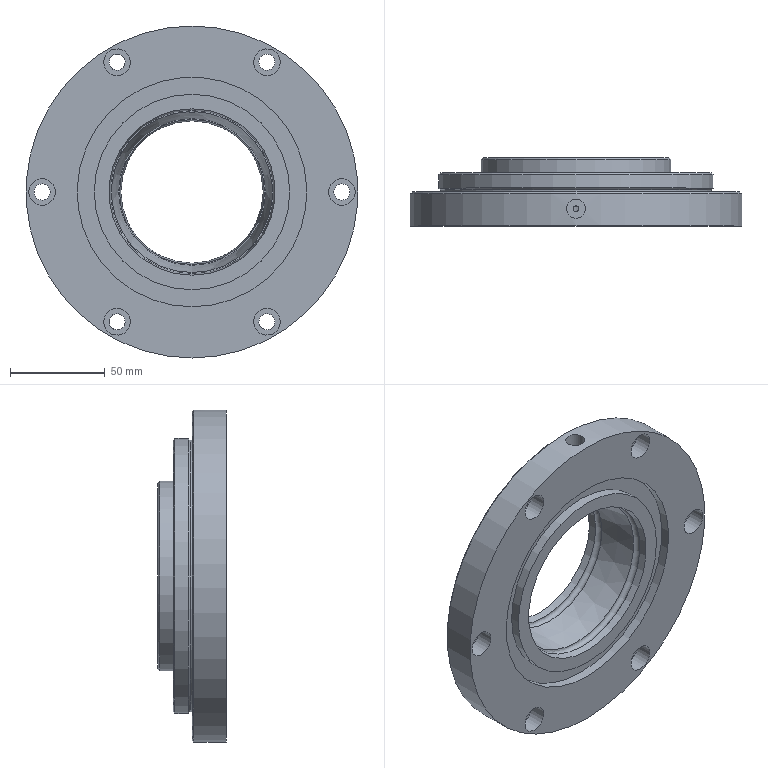Part | NX | features IDENTICAL INSTANCE OUTPUT 5, Instance Feature 5, DATUM_CSYS 3, CBORE_HOLE 2, HOLE PACKAGE 2, SKETCH 2, CHAMFER 1, MASTER SNAPSHOT BODY 1, Pattern Feature 1, SWP104 1 | 1 solid | 44 faces | box 175 x 36 x 175 mm | volume 439524 mm3 | cylinder 20 | plane 14 | cone 8 | torus 2 | commonest cylinder face diameters 8.5 x6 14 x6 3 x1 10 x1 100 x1 103 x1
STEP:
#1=CARTESIAN_POINT('',(0.,0.,-43.848));
#2=VERTEX_POINT('',#1);
#3=CARTESIAN_POINT('',(0.,0.,0.));
#4=DIRECTION('',(0.,-1.,0.));
#5=DIRECTION('',(0.,0.,-1.));
#6=AXIS2_PLACEMENT_3D('',#3,#4,#5);
#7=CIRCLE('',#6,43.848);
#8=EDGE_CURVE('',#2,#2,#7,.T.);
#9=ORIENTED_EDGE('',*,*,#8,.F.);
#10=EDGE_LOOP('',(#9));
#11=FACE_BOUND('',#10,.T.);
#12=CARTESIAN_POINT('',(0.,0.,-51.5));
#13=VERTEX_POINT('',#12);
#14=CARTESIAN_POINT('',(0.,0.,0.));
#15=DIRECTION('',(0.,-1.,0.));
#16=DIRECTION('',(0.,0.,-1.));
#17=AXIS2_PLACEMENT_3D('',#14,#15,#16);
#18=CIRCLE('',#17,51.5);
#19=EDGE_CURVE('',#13,#13,#18,.T.);
#20=ORIENTED_EDGE('',*,*,#19,.T.);
#21=EDGE_LOOP('',(#20));
#22=FACE_BOUND('',#21,.T.);
#23=CARTESIAN_POINT('',(0.,0.,51.5));
#24=DIRECTION('',(0.,1.,0.));
#25=DIRECTION('',(0.,0.,1.));
#26=AXIS2_PLACEMENT_3D('',#23,#24,#25);
#27=PLANE('',#26);
#28=ADVANCED_FACE('',(#11,#22),#27,.F.);
#29=CARTESIAN_POINT('',(0.,4.,-43.142));
#30=VERTEX_POINT('',#29);
#31=CARTESIAN_POINT('',(0.,4.,0.));
#32=DIRECTION('',(0.,-1.,0.));
#33=DIRECTION('',(0.,0.,-1.));
#34=AXIS2_PLACEMENT_3D('',#31,#32,#33);
#35=CIRCLE('',#34,43.142);
#36=EDGE_CURVE('',#30,#30,#35,.T.);
#37=ORIENTED_EDGE('',*,*,#36,.F.);
#38=EDGE_LOOP('',(#37));
#39=FACE_BOUND('',#38,.T.);
#40=ORIENTED_EDGE('',*,*,#8,.T.);
#41=EDGE_LOOP('',(#40));
#42=FACE_BOUND('',#41,.T.);
#43=CARTESIAN_POINT('',(0.,0.,0.));
#44=DIRECTION('',(0.,-1.,0.));
#45=DIRECTION('',(0.,0.,-1.));
#46=AXIS2_PLACEMENT_3D('',#43,#44,#45);
#47=CONICAL_SURFACE('',#46,43.848,0.1745);
#48=ADVANCED_FACE('',(#39,#42),#47,.F.);
#49=CARTESIAN_POINT('',(-1.061,7.939,42.435));
#50=VERTEX_POINT('',#49);
#51=CARTESIAN_POINT('',(1.061,7.939,42.435));
#52=VERTEX_POINT('',#51);
#53=CARTESIAN_POINT('',(0.,7.939,0.));
#54=DIRECTION('',(0.,-1.,0.));
#55=DIRECTION('',(0.,0.,-1.));
#56=AXIS2_PLACEMENT_3D('',#53,#54,#55);
#57=CIRCLE('',#56,42.448);
#58=EDGE_CURVE('',#50,#52,#57,.T.);
#59=ORIENTED_EDGE('',*,*,#58,.F.);
#60=CARTESIAN_POINT('',(-1.061,7.939,42.435));
#61=CARTESIAN_POINT('',(-1.128,8.006,42.814));
#62=CARTESIAN_POINT('',(-1.087,7.877,43.66));
#63=CARTESIAN_POINT('',(-0.2099,7.412,44.182));
#64=CARTESIAN_POINT('',(0.5847,7.583,43.99));
#65=CARTESIAN_POINT('',(1.08,7.916,43.444));
#66=CARTESIAN_POINT('',(1.128,8.006,42.814));
#67=CARTESIAN_POINT('',(1.061,7.939,42.435));
#68=B_SPLINE_CURVE_WITH_KNOTS('',3,(#60,#61,#62,#63,#64,#65,#66,#67),.UNSPECIFIED.,.F.,.F.,(4,1,1,1,1,4),(0.0008258,0.001986,0.003146,0.003726,0.004307,0.005467),.UNSPECIFIED.);
#69=EDGE_CURVE('',#50,#52,#68,.T.);
#70=ORIENTED_EDGE('',*,*,#69,.T.);
#71=EDGE_LOOP('',(#59,#70));
#72=FACE_BOUND('',#71,.T.);
#73=ORIENTED_EDGE('',*,*,#36,.T.);
#74=EDGE_LOOP('',(#73));
#75=FACE_BOUND('',#74,.T.);
#76=CARTESIAN_POINT('',(0.,5.97,0.));
#77=DIRECTION('',(0.,-1.,0.));
#78=DIRECTION('',(0.,0.,-1.));
#79=AXIS2_PLACEMENT_3D('',#76,#77,#78);
#80=TOROIDAL_SURFACE('',#79,42.795,2.);
#81=ADVANCED_FACE('',(#72,#75),#80,.F.);
#82=CARTESIAN_POINT('',(0.,28.061,-38.9));
#83=VERTEX_POINT('',#82);
#84=CARTESIAN_POINT('',(0.,28.061,0.));
#85=DIRECTION('',(0.,-1.,0.));
#86=DIRECTION('',(0.,0.,-1.));
#87=AXIS2_PLACEMENT_3D('',#84,#85,#86);
#88=CIRCLE('',#87,38.9);
#89=EDGE_CURVE('',#83,#83,#88,.T.);
#90=ORIENTED_EDGE('',*,*,#89,.F.);
#91=EDGE_LOOP('',(#90));
#92=FACE_BOUND('',#91,.T.);
#93=ORIENTED_EDGE('',*,*,#58,.T.);
#94=CARTESIAN_POINT('',(1.061,7.939,42.435));
#95=CARTESIAN_POINT('',(1.481,8.359,42.35));
#96=CARTESIAN_POINT('',(1.747,9.702,42.103));
#97=CARTESIAN_POINT('',(0.001721,10.899,41.943));
#98=CARTESIAN_POINT('',(-1.747,9.703,42.103));
#99=CARTESIAN_POINT('',(-1.481,8.359,42.35));
#100=CARTESIAN_POINT('',(-1.061,7.939,42.435));
#101=B_SPLINE_CURVE_WITH_KNOTS('',3,(#94,#95,#96,#97,#98,#99,#100),.UNSPECIFIED.,.F.,.F.,(4,1,1,1,4),(0.000000282,0.001775,0.003549,0.005324,0.007098),.UNSPECIFIED.);
#102=EDGE_CURVE('',#52,#50,#101,.T.);
#103=ORIENTED_EDGE('',*,*,#102,.T.);
#104=EDGE_LOOP('',(#93,#103));
#105=FACE_BOUND('',#104,.T.);
#106=CARTESIAN_POINT('',(0.,7.939,0.));
#107=DIRECTION('',(0.,-1.,0.));
#108=DIRECTION('',(0.,0.,-1.));
#109=AXIS2_PLACEMENT_3D('',#106,#107,#108);
#110=CONICAL_SURFACE('',#109,42.448,0.1745);
#111=ADVANCED_FACE('',(#92,#105),#110,.F.);
#112=CARTESIAN_POINT('',(0.,32.,-38.205));
#113=VERTEX_POINT('',#112);
#114=CARTESIAN_POINT('',(0.,32.,0.));
#115=DIRECTION('',(0.,-1.,0.));
#116=DIRECTION('',(0.,0.,-1.));
#117=AXIS2_PLACEMENT_3D('',#114,#115,#116);
#118=CIRCLE('',#117,38.205);
#119=EDGE_CURVE('',#113,#113,#118,.T.);
#120=ORIENTED_EDGE('',*,*,#119,.F.);
#121=EDGE_LOOP('',(#120));
#122=FACE_BOUND('',#121,.T.);
#123=ORIENTED_EDGE('',*,*,#89,.T.);
#124=EDGE_LOOP('',(#123));
#125=FACE_BOUND('',#124,.T.);
#126=CARTESIAN_POINT('',(0.,30.03,0.));
#127=DIRECTION('',(0.,-1.,0.));
#128=DIRECTION('',(0.,0.,-1.));
#129=AXIS2_PLACEMENT_3D('',#126,#127,#128);
#130=TOROIDAL_SURFACE('',#129,38.553,2.);
#131=ADVANCED_FACE('',(#122,#125),#130,.F.);
#132=CARTESIAN_POINT('',(0.,36.,-37.5));
#133=VERTEX_POINT('',#132);
#134=CARTESIAN_POINT('',(0.,36.,0.));
#135=DIRECTION('',(0.,-1.,0.));
#136=DIRECTION('',(0.,0.,-1.));
#137=AXIS2_PLACEMENT_3D('',#134,#135,#136);
#138=CIRCLE('',#137,37.5);
#139=EDGE_CURVE('',#133,#133,#138,.T.);
#140=ORIENTED_EDGE('',*,*,#139,.F.);
#141=EDGE_LOOP('',(#140));
#142=FACE_BOUND('',#141,.T.);
#143=ORIENTED_EDGE('',*,*,#119,.T.);
#144=EDGE_LOOP('',(#143));
#145=FACE_BOUND('',#144,.T.);
#146=CARTESIAN_POINT('',(0.,32.,0.));
#147=DIRECTION('',(0.,-1.,0.));
#148=DIRECTION('',(0.,0.,-1.));
#149=AXIS2_PLACEMENT_3D('',#146,#147,#148);
#150=CONICAL_SURFACE('',#149,38.205,0.1745);
#151=ADVANCED_FACE('',(#142,#145),#150,.F.);
#152=CARTESIAN_POINT('',(0.,36.,-49.));
#153=VERTEX_POINT('',#152);
#154=CARTESIAN_POINT('',(0.,36.,0.));
#155=DIRECTION('',(0.,-1.,0.));
#156=DIRECTION('',(0.,0.,-1.));
#157=AXIS2_PLACEMENT_3D('',#154,#155,#156);
#158=CIRCLE('',#157,49.);
#159=EDGE_CURVE('',#153,#153,#158,.F.);
#160=ORIENTED_EDGE('',*,*,#159,.T.);
#161=EDGE_LOOP('',(#160));
#162=FACE_BOUND('',#161,.T.);
#163=ORIENTED_EDGE('',*,*,#139,.T.);
#164=EDGE_LOOP('',(#163));
#165=FACE_BOUND('',#164,.T.);
#166=CARTESIAN_POINT('',(0.,36.,37.5));
#167=DIRECTION('',(0.,-1.,0.));
#168=DIRECTION('',(0.,0.,-1.));
#169=AXIS2_PLACEMENT_3D('',#166,#167,#168);
#170=PLANE('',#169);
#171=ADVANCED_FACE('',(#162,#165),#170,.F.);
#172=CARTESIAN_POINT('',(0.,35.,-50.));
#173=VERTEX_POINT('',#172);
#174=CARTESIAN_POINT('',(0.,35.,0.));
#175=DIRECTION('',(0.,-1.,0.));
#176=DIRECTION('',(0.,0.,-1.));
#177=AXIS2_PLACEMENT_3D('',#174,#175,#176);
#178=CIRCLE('',#177,50.);
#179=EDGE_CURVE('',#173,#173,#178,.T.);
#180=ORIENTED_EDGE('',*,*,#179,.T.);
#181=EDGE_LOOP('',(#180));
#182=FACE_BOUND('',#181,.T.);
#183=CARTESIAN_POINT('',(0.,28.,-50.));
#184=VERTEX_POINT('',#183);
#185=CARTESIAN_POINT('',(0.,28.,0.));
#186=DIRECTION('',(0.,-1.,0.));
#187=DIRECTION('',(0.,0.,-1.));
#188=AXIS2_PLACEMENT_3D('',#185,#186,#187);
#189=CIRCLE('',#188,50.);
#190=EDGE_CURVE('',#184,#184,#189,.T.);
#191=ORIENTED_EDGE('',*,*,#190,.F.);
#192=EDGE_LOOP('',(#191));
#193=FACE_BOUND('',#192,.T.);
#194=CARTESIAN_POINT('',(0.,0.,0.));
#195=DIRECTION('',(0.,-1.,0.));
#196=DIRECTION('',(0.,0.,-1.));
#197=AXIS2_PLACEMENT_3D('',#194,#195,#196);
#198=CYLINDRICAL_SURFACE('',#197,50.);
#199=ADVANCED_FACE('',(#182,#193),#198,.T.);
#200=CARTESIAN_POINT('',(0.,28.,-71.5));
#201=VERTEX_POINT('',#200);
#202=CARTESIAN_POINT('',(0.,28.,0.));
#203=DIRECTION('',(0.,-1.,0.));
#204=DIRECTION('',(0.,0.,-1.));
#205=AXIS2_PLACEMENT_3D('',#202,#203,#204);
#206=CIRCLE('',#205,71.5);
#207=EDGE_CURVE('',#201,#201,#206,.F.);
#208=ORIENTED_EDGE('',*,*,#207,.T.);
#209=EDGE_LOOP('',(#208));
#210=FACE_BOUND('',#209,.T.);
#211=ORIENTED_EDGE('',*,*,#190,.T.);
#212=EDGE_LOOP('',(#211));
#213=FACE_BOUND('',#212,.T.);
#214=CARTESIAN_POINT('',(0.,28.,50.));
#215=DIRECTION('',(0.,-1.,0.));
#216=DIRECTION('',(0.,0.,-1.));
#217=AXIS2_PLACEMENT_3D('',#214,#215,#216);
#218=PLANE('',#217);
#219=ADVANCED_FACE('',(#210,#213),#218,.F.);
#220=CARTESIAN_POINT('',(0.,27.,-72.5));
#221=VERTEX_POINT('',#220);
#222=CARTESIAN_POINT('',(0.,27.,0.));
#223=DIRECTION('',(0.,-1.,0.));
#224=DIRECTION('',(0.,0.,-1.));
#225=AXIS2_PLACEMENT_3D('',#222,#223,#224);
#226=CIRCLE('',#225,72.5);
#227=EDGE_CURVE('',#221,#221,#226,.T.);
#228=ORIENTED_EDGE('',*,*,#227,.T.);
#229=EDGE_LOOP('',(#228));
#230=FACE_BOUND('',#229,.T.);
#231=CARTESIAN_POINT('',(0.,20.,-72.5));
#232=VERTEX_POINT('',#231);
#233=CARTESIAN_POINT('',(0.,20.,0.));
#234=DIRECTION('',(0.,-1.,0.));
#235=DIRECTION('',(0.,0.,-1.));
#236=AXIS2_PLACEMENT_3D('',#233,#234,#235);
#237=CIRCLE('',#236,72.5);
#238=EDGE_CURVE('',#232,#232,#237,.T.);
#239=ORIENTED_EDGE('',*,*,#238,.F.);
#240=EDGE_LOOP('',(#239));
#241=FACE_BOUND('',#240,.T.);
#242=CARTESIAN_POINT('',(0.,0.,0.));
#243=DIRECTION('',(0.,-1.,0.));
#244=DIRECTION('',(0.,0.,-1.));
#245=AXIS2_PLACEMENT_3D('',#242,#243,#244);
#246=CYLINDRICAL_SURFACE('',#245,72.5);
#247=ADVANCED_FACE('',(#230,#241),#246,.T.);
#248=CARTESIAN_POINT('',(0.,19.,-71.5));
#249=VERTEX_POINT('',#248);
#250=CARTESIAN_POINT('',(0.,19.,0.));
#251=DIRECTION('',(0.,-1.,0.));
#252=DIRECTION('',(0.,0.,-1.));
#253=AXIS2_PLACEMENT_3D('',#250,#251,#252);
#254=CIRCLE('',#253,71.5);
#255=EDGE_CURVE('',#249,#249,#254,.T.);
#256=ORIENTED_EDGE('',*,*,#255,.F.);
#257=EDGE_LOOP('',(#256));
#258=FACE_BOUND('',#257,.T.);
#259=ORIENTED_EDGE('',*,*,#238,.T.);
#260=EDGE_LOOP('',(#259));
#261=FACE_BOUND('',#260,.T.);
#262=CARTESIAN_POINT('',(0.,20.,0.));
#263=DIRECTION('',(0.,1.,0.));
#264=DIRECTION('',(0.,0.,1.));
#265=AXIS2_PLACEMENT_3D('',#262,#263,#264);
#266=CONICAL_SURFACE('',#265,72.5,0.7854);
#267=ADVANCED_FACE('',(#258,#261),#266,.T.);
#268=CARTESIAN_POINT('',(0.,17.,-71.5));
#269=VERTEX_POINT('',#268);
#270=CARTESIAN_POINT('',(0.,17.,0.));
#271=DIRECTION('',(0.,-1.,0.));
#272=DIRECTION('',(0.,0.,-1.));
#273=AXIS2_PLACEMENT_3D('',#270,#271,#272);
#274=CIRCLE('',#273,71.5);
#275=EDGE_CURVE('',#269,#269,#274,.T.);
#276=ORIENTED_EDGE('',*,*,#275,.F.);
#277=EDGE_LOOP('',(#276));
#278=FACE_BOUND('',#277,.T.);
#279=ORIENTED_EDGE('',*,*,#255,.T.);
#280=EDGE_LOOP('',(#279));
#281=FACE_BOUND('',#280,.T.);
#282=CARTESIAN_POINT('',(0.,0.,0.));
#283=DIRECTION('',(0.,-1.,0.));
#284=DIRECTION('',(0.,0.,-1.));
#285=AXIS2_PLACEMENT_3D('',#282,#283,#284);
#286=CYLINDRICAL_SURFACE('',#285,71.5);
#287=ADVANCED_FACE('',(#278,#281),#286,.T.);
#288=CARTESIAN_POINT('',(0.,17.,-73.));
#289=VERTEX_POINT('',#288);
#290=CARTESIAN_POINT('',(0.,17.,0.));
#291=DIRECTION('',(0.,-1.,0.));
#292=DIRECTION('',(0.,0.,-1.));
#293=AXIS2_PLACEMENT_3D('',#290,#291,#292);
#294=CIRCLE('',#293,73.);
#295=EDGE_CURVE('',#289,#289,#294,.T.);
#296=ORIENTED_EDGE('',*,*,#295,.F.);
#297=EDGE_LOOP('',(#296));
#298=FACE_BOUND('',#297,.T.);
#299=ORIENTED_EDGE('',*,*,#275,.T.);
#300=EDGE_LOOP('',(#299));
#301=FACE_BOUND('',#300,.T.);
#302=CARTESIAN_POINT('',(0.,17.,71.5));
#303=DIRECTION('',(0.,-1.,0.));
#304=DIRECTION('',(0.,0.,-1.));
#305=AXIS2_PLACEMENT_3D('',#302,#303,#304);
#306=PLANE('',#305);
#307=ADVANCED_FACE('',(#298,#301),#306,.F.);
#308=CARTESIAN_POINT('',(0.,18.,-74.));
#309=VERTEX_POINT('',#308);
#310=CARTESIAN_POINT('',(0.,18.,0.));
#311=DIRECTION('',(0.,-1.,0.));
#312=DIRECTION('',(0.,0.,-1.));
#313=AXIS2_PLACEMENT_3D('',#310,#311,#312);
#314=CIRCLE('',#313,74.);
#315=EDGE_CURVE('',#309,#309,#314,.T.);
#316=ORIENTED_EDGE('',*,*,#315,.F.);
#317=EDGE_LOOP('',(#316));
#318=FACE_BOUND('',#317,.T.);
#319=ORIENTED_EDGE('',*,*,#295,.T.);
#320=EDGE_LOOP('',(#319));
#321=FACE_BOUND('',#320,.T.);
#322=CARTESIAN_POINT('',(0.,17.,0.));
#323=DIRECTION('',(0.,1.,0.));
#324=DIRECTION('',(0.,0.,1.));
#325=AXIS2_PLACEMENT_3D('',#322,#323,#324);
#326=CONICAL_SURFACE('',#325,73.,0.7854);
#327=ADVANCED_FACE('',(#318,#321),#326,.F.);
#328=CARTESIAN_POINT('',(39.5,18.,-72.666));
#329=VERTEX_POINT('',#328);
#330=CARTESIAN_POINT('',(39.5,18.,-68.416));
#331=DIRECTION('',(0.,-1.,0.));
#332=DIRECTION('',(0.,0.,-1.));
#333=AXIS2_PLACEMENT_3D('',#330,#331,#332);
#334=CIRCLE('',#333,4.25);
#335=EDGE_CURVE('',#329,#329,#334,.T.);
#336=ORIENTED_EDGE('',*,*,#335,.T.);
#337=EDGE_LOOP('',(#336));
#338=FACE_BOUND('',#337,.T.);
#339=CARTESIAN_POINT('',(-39.5,18.,-72.666));
#340=VERTEX_POINT('',#339);
#341=CARTESIAN_POINT('',(-39.5,18.,-68.416));
#342=DIRECTION('',(0.,-1.,0.));
#343=DIRECTION('',(0.,0.,-1.));
#344=AXIS2_PLACEMENT_3D('',#341,#342,#343);
#345=CIRCLE('',#344,4.25);
#346=EDGE_CURVE('',#340,#340,#345,.T.);
#347=ORIENTED_EDGE('',*,*,#346,.T.);
#348=EDGE_LOOP('',(#347));
#349=FACE_BOUND('',#348,.T.);
#350=CARTESIAN_POINT('',(-79.,18.,-4.25));
#351=VERTEX_POINT('',#350);
#352=CARTESIAN_POINT('',(-79.,18.,0.));
#353=DIRECTION('',(0.,-1.,0.));
#354=DIRECTION('',(0.,0.,-1.));
#355=AXIS2_PLACEMENT_3D('',#352,#353,#354);
#356=CIRCLE('',#355,4.25);
#357=EDGE_CURVE('',#351,#351,#356,.T.);
#358=ORIENTED_EDGE('',*,*,#357,.T.);
#359=EDGE_LOOP('',(#358));
#360=FACE_BOUND('',#359,.T.);
#361=CARTESIAN_POINT('',(-39.5,18.,64.166));
#362=VERTEX_POINT('',#361);
#363=CARTESIAN_POINT('',(-39.5,18.,68.416));
#364=DIRECTION('',(0.,-1.,0.));
#365=DIRECTION('',(0.,0.,-1.));
#366=AXIS2_PLACEMENT_3D('',#363,#364,#365);
#367=CIRCLE('',#366,4.25);
#368=EDGE_CURVE('',#362,#362,#367,.T.);
#369=ORIENTED_EDGE('',*,*,#368,.T.);
#370=EDGE_LOOP('',(#369));
#371=FACE_BOUND('',#370,.T.);
#372=CARTESIAN_POINT('',(39.5,18.,64.166));
#373=VERTEX_POINT('',#372);
#374=CARTESIAN_POINT('',(39.5,18.,68.416));
#375=DIRECTION('',(0.,-1.,0.));
#376=DIRECTION('',(0.,0.,-1.));
#377=AXIS2_PLACEMENT_3D('',#374,#375,#376);
#378=CIRCLE('',#377,4.25);
#379=EDGE_CURVE('',#373,#373,#378,.T.);
#380=ORIENTED_EDGE('',*,*,#379,.T.);
#381=EDGE_LOOP('',(#380));
#382=FACE_BOUND('',#381,.T.);
#383=CARTESIAN_POINT('',(79.,18.,-4.25));
#384=VERTEX_POINT('',#383);
#385=CARTESIAN_POINT('',(79.,18.,0.));
#386=DIRECTION('',(0.,-1.,0.));
#387=DIRECTION('',(0.,0.,-1.));
#388=AXIS2_PLACEMENT_3D('',#385,#386,#387);
#389=CIRCLE('',#388,4.25);
#390=EDGE_CURVE('',#384,#384,#389,.T.);
#391=ORIENTED_EDGE('',*,*,#390,.T.);
#392=EDGE_LOOP('',(#391));
#393=FACE_BOUND('',#392,.T.);
#394=CARTESIAN_POINT('',(0.,18.,-86.5));
#395=VERTEX_POINT('',#394);
#396=CARTESIAN_POINT('',(0.,18.,0.));
#397=DIRECTION('',(0.,-1.,0.));
#398=DIRECTION('',(0.,0.,-1.));
#399=AXIS2_PLACEMENT_3D('',#396,#397,#398);
#400=CIRCLE('',#399,86.5);
#401=EDGE_CURVE('',#395,#395,#400,.F.);
#402=ORIENTED_EDGE('',*,*,#401,.T.);
#403=EDGE_LOOP('',(#402));
#404=FACE_BOUND('',#403,.T.);
#405=ORIENTED_EDGE('',*,*,#315,.T.);
#406=EDGE_LOOP('',(#405));
#407=FACE_BOUND('',#406,.T.);
#408=CARTESIAN_POINT('',(0.,18.,74.));
#409=DIRECTION('',(0.,-1.,0.));
#410=DIRECTION('',(0.,0.,-1.));
#411=AXIS2_PLACEMENT_3D('',#408,#409,#410);
#412=PLANE('',#411);
#413=ADVANCED_FACE('',(#338,#349,#360,#371,#382,#393,#404,#407),#412,.F.);
#414=CARTESIAN_POINT('',(0.,17.,-87.5));
#415=VERTEX_POINT('',#414);
#416=CARTESIAN_POINT('',(0.,17.,0.));
#417=DIRECTION('',(0.,-1.,0.));
#418=DIRECTION('',(0.,0.,-1.));
#419=AXIS2_PLACEMENT_3D('',#416,#417,#418);
#420=CIRCLE('',#419,87.5);
#421=EDGE_CURVE('',#415,#415,#420,.T.);
#422=ORIENTED_EDGE('',*,*,#421,.T.);
#423=EDGE_LOOP('',(#422));
#424=FACE_BOUND('',#423,.T.);
#425=CARTESIAN_POINT('',(-5.,9.,87.357));
#426=VERTEX_POINT('',#425);
#427=CARTESIAN_POINT('',(-3.915,5.078,87.429));
#428=CARTESIAN_POINT('',(-5.542,9.001,87.321));
#429=CARTESIAN_POINT('',(-3.916,12.918,87.429));
#430=CARTESIAN_POINT('',(-0.004129,14.54,87.536));
#431=CARTESIAN_POINT('',(3.917,12.921,87.429));
#432=CARTESIAN_POINT('',(5.54,9.001,87.321));
#433=CARTESIAN_POINT('',(3.922,5.087,87.428));
#434=CARTESIAN_POINT('',(0.005768,3.459,87.536));
#435=CARTESIAN_POINT('',(-3.915,5.078,87.429));
#436=CARTESIAN_POINT('',(-5.542,9.001,87.321));
#437=CARTESIAN_POINT('',(-3.916,12.918,87.429));
#438=B_SPLINE_CURVE_WITH_KNOTS('',3,(#427,#428,#429,#430,#431,#432,#433,#434,#435,#436,#437),.UNSPECIFIED.,.T.,.F.,(1,1,1,1,1,1,1,1,1,1,1,1,1,1,1),(-0.01173,-0.007817,-0.003908,0.,0.003908,0.007817,0.01173,0.01563,0.01954,0.02345,0.02736,0.03127,0.03518,0.03908,0.04299),.UNSPECIFIED.);
#439=EDGE_CURVE('',#426,#426,#438,.T.);
#440=ORIENTED_EDGE('',*,*,#439,.T.);
#441=EDGE_LOOP('',(#440));
#442=FACE_BOUND('',#441,.T.);
#443=CARTESIAN_POINT('',(0.,0.,-87.5));
#444=VERTEX_POINT('',#443);
#445=CARTESIAN_POINT('',(0.,0.,0.));
#446=DIRECTION('',(0.,-1.,0.));
#447=DIRECTION('',(0.,0.,-1.));
#448=AXIS2_PLACEMENT_3D('',#445,#446,#447);
#449=CIRCLE('',#448,87.5);
#450=EDGE_CURVE('',#444,#444,#449,.T.);
#451=ORIENTED_EDGE('',*,*,#450,.F.);
#452=EDGE_LOOP('',(#451));
#453=FACE_BOUND('',#452,.T.);
#454=CARTESIAN_POINT('',(0.,0.,0.));
#455=DIRECTION('',(0.,-1.,0.));
#456=DIRECTION('',(0.,0.,-1.));
#457=AXIS2_PLACEMENT_3D('',#454,#455,#456);
#458=CYLINDRICAL_SURFACE('',#457,87.5);
#459=ADVANCED_FACE('',(#424,#442,#453),#458,.T.);
#460=CARTESIAN_POINT('',(45.562,0.,-64.916));
#461=VERTEX_POINT('',#460);
#462=CARTESIAN_POINT('',(39.5,0.,-68.416));
#463=DIRECTION('',(0.,1.,0.));
#464=DIRECTION('',(0.866,0.,0.5));
#465=AXIS2_PLACEMENT_3D('',#462,#463,#464);
#466=CIRCLE('',#465,7.);
#467=EDGE_CURVE('',#461,#461,#466,.T.);
#468=ORIENTED_EDGE('',*,*,#467,.T.);
#469=EDGE_LOOP('',(#468));
#470=FACE_BOUND('',#469,.T.);
#471=CARTESIAN_POINT('',(-33.438,0.,-71.916));
#472=VERTEX_POINT('',#471);
#473=CARTESIAN_POINT('',(-39.5,0.,-68.416));
#474=DIRECTION('',(0.,1.,0.));
#475=DIRECTION('',(0.866,0.,-0.5));
#476=AXIS2_PLACEMENT_3D('',#473,#474,#475);
#477=CIRCLE('',#476,7.);
#478=EDGE_CURVE('',#472,#472,#477,.T.);
#479=ORIENTED_EDGE('',*,*,#478,.T.);
#480=EDGE_LOOP('',(#479));
#481=FACE_BOUND('',#480,.T.);
#482=CARTESIAN_POINT('',(-79.,0.,-7.));
#483=VERTEX_POINT('',#482);
#484=CARTESIAN_POINT('',(-79.,0.,0.));
#485=DIRECTION('',(0.,1.,0.));
#486=DIRECTION('',(0.,0.,-1.));
#487=AXIS2_PLACEMENT_3D('',#484,#485,#486);
#488=CIRCLE('',#487,7.);
#489=EDGE_CURVE('',#483,#483,#488,.T.);
#490=ORIENTED_EDGE('',*,*,#489,.T.);
#491=EDGE_LOOP('',(#490));
#492=FACE_BOUND('',#491,.T.);
#493=CARTESIAN_POINT('',(-45.562,0.,64.916));
#494=VERTEX_POINT('',#493);
#495=CARTESIAN_POINT('',(-39.5,0.,68.416));
#496=DIRECTION('',(0.,1.,0.));
#497=DIRECTION('',(-0.866,0.,-0.5));
#498=AXIS2_PLACEMENT_3D('',#495,#496,#497);
#499=CIRCLE('',#498,7.);
#500=EDGE_CURVE('',#494,#494,#499,.T.);
#501=ORIENTED_EDGE('',*,*,#500,.T.);
#502=EDGE_LOOP('',(#501));
#503=FACE_BOUND('',#502,.T.);
#504=CARTESIAN_POINT('',(33.438,0.,71.916));
#505=VERTEX_POINT('',#504);
#506=CARTESIAN_POINT('',(39.5,0.,68.416));
#507=DIRECTION('',(0.,1.,0.));
#508=DIRECTION('',(-0.866,0.,0.5));
#509=AXIS2_PLACEMENT_3D('',#506,#507,#508);
#510=CIRCLE('',#509,7.);
#511=EDGE_CURVE('',#505,#505,#510,.T.);
#512=ORIENTED_EDGE('',*,*,#511,.T.);
#513=EDGE_LOOP('',(#512));
#514=FACE_BOUND('',#513,.T.);
#515=CARTESIAN_POINT('',(79.,0.,7.));
#516=VERTEX_POINT('',#515);
#517=CARTESIAN_POINT('',(79.,0.,0.));
#518=DIRECTION('',(0.,1.,0.));
#519=DIRECTION('',(0.,0.,1.));
#520=AXIS2_PLACEMENT_3D('',#517,#518,#519);
#521=CIRCLE('',#520,7.);
#522=EDGE_CURVE('',#516,#516,#521,.T.);
#523=ORIENTED_EDGE('',*,*,#522,.T.);
#524=EDGE_LOOP('',(#523));
#525=FACE_BOUND('',#524,.T.);
#526=CARTESIAN_POINT('',(0.,0.,-60.5));
#527=VERTEX_POINT('',#526);
#528=CARTESIAN_POINT('',(0.,0.,0.));
#529=DIRECTION('',(0.,-1.,0.));
#530=DIRECTION('',(0.,0.,-1.));
#531=AXIS2_PLACEMENT_3D('',#528,#529,#530);
#532=CIRCLE('',#531,60.5);
#533=EDGE_CURVE('',#527,#527,#532,.T.);
#534=ORIENTED_EDGE('',*,*,#533,.F.);
#535=EDGE_LOOP('',(#534));
#536=FACE_BOUND('',#535,.T.);
#537=ORIENTED_EDGE('',*,*,#450,.T.);
#538=EDGE_LOOP('',(#537));
#539=FACE_BOUND('',#538,.T.);
#540=CARTESIAN_POINT('',(0.,0.,87.5));
#541=DIRECTION('',(0.,1.,0.));
#542=DIRECTION('',(0.,0.,1.));
#543=AXIS2_PLACEMENT_3D('',#540,#541,#542);
#544=PLANE('',#543);
#545=ADVANCED_FACE('',(#470,#481,#492,#503,#514,#525,#536,#539),#544,.F.);
#546=CARTESIAN_POINT('',(0.,5.,-60.5));
#547=VERTEX_POINT('',#546);
#548=CARTESIAN_POINT('',(0.,5.,0.));
#549=DIRECTION('',(0.,-1.,0.));
#550=DIRECTION('',(0.,0.,-1.));
#551=AXIS2_PLACEMENT_3D('',#548,#549,#550);
#552=CIRCLE('',#551,60.5);
#553=EDGE_CURVE('',#547,#547,#552,.T.);
#554=ORIENTED_EDGE('',*,*,#553,.F.);
#555=EDGE_LOOP('',(#554));
#556=FACE_BOUND('',#555,.T.);
#557=ORIENTED_EDGE('',*,*,#533,.T.);
#558=EDGE_LOOP('',(#557));
#559=FACE_BOUND('',#558,.T.);
#560=CARTESIAN_POINT('',(0.,0.,0.));
#561=DIRECTION('',(0.,-1.,0.));
#562=DIRECTION('',(0.,0.,-1.));
#563=AXIS2_PLACEMENT_3D('',#560,#561,#562);
#564=CYLINDRICAL_SURFACE('',#563,60.5);
#565=ADVANCED_FACE('',(#556,#559),#564,.F.);
#566=CARTESIAN_POINT('',(0.,5.,-51.5));
#567=VERTEX_POINT('',#566);
#568=CARTESIAN_POINT('',(0.,5.,0.));
#569=DIRECTION('',(0.,-1.,0.));
#570=DIRECTION('',(0.,0.,-1.));
#571=AXIS2_PLACEMENT_3D('',#568,#569,#570);
#572=CIRCLE('',#571,51.5);
#573=EDGE_CURVE('',#567,#567,#572,.T.);
#574=ORIENTED_EDGE('',*,*,#573,.F.);
#575=EDGE_LOOP('',(#574));
#576=FACE_BOUND('',#575,.T.);
#577=ORIENTED_EDGE('',*,*,#553,.T.);
#578=EDGE_LOOP('',(#577));
#579=FACE_BOUND('',#578,.T.);
#580=CARTESIAN_POINT('',(0.,5.,60.5));
#581=DIRECTION('',(0.,1.,0.));
#582=DIRECTION('',(0.,0.,1.));
#583=AXIS2_PLACEMENT_3D('',#580,#581,#582);
#584=PLANE('',#583);
#585=ADVANCED_FACE('',(#576,#579),#584,.F.);
#586=ORIENTED_EDGE('',*,*,#19,.F.);
#587=EDGE_LOOP('',(#586));
#588=FACE_BOUND('',#587,.T.);
#589=ORIENTED_EDGE('',*,*,#573,.T.);
#590=EDGE_LOOP('',(#589));
#591=FACE_BOUND('',#590,.T.);
#592=CARTESIAN_POINT('',(0.,0.,0.));
#593=DIRECTION('',(0.,-1.,0.));
#594=DIRECTION('',(0.,0.,-1.));
#595=AXIS2_PLACEMENT_3D('',#592,#593,#594);
#596=CYLINDRICAL_SURFACE('',#595,51.5);
#597=ADVANCED_FACE('',(#588,#591),#596,.T.);
#598=CARTESIAN_POINT('',(-5.,9.,75.5));
#599=VERTEX_POINT('',#598);
#600=CARTESIAN_POINT('',(0.,9.,75.5));
#601=DIRECTION('',(0.,0.,-1.));
#602=DIRECTION('',(-1.,0.,0.));
#603=AXIS2_PLACEMENT_3D('',#600,#601,#602);
#604=CIRCLE('',#603,5.);
#605=EDGE_CURVE('',#599,#599,#604,.F.);
#606=ORIENTED_EDGE('',*,*,#605,.F.);
#607=EDGE_LOOP('',(#606));
#608=FACE_BOUND('',#607,.T.);
#609=ORIENTED_EDGE('',*,*,#439,.F.);
#610=EDGE_LOOP('',(#609));
#611=FACE_BOUND('',#610,.T.);
#612=CARTESIAN_POINT('',(0.,9.,87.5));
#613=DIRECTION('',(0.,0.,-1.));
#614=DIRECTION('',(-1.,0.,0.));
#615=AXIS2_PLACEMENT_3D('',#612,#613,#614);
#616=CYLINDRICAL_SURFACE('',#615,5.);
#617=ADVANCED_FACE('',(#608,#611),#616,.F.);
#618=CARTESIAN_POINT('',(-1.5,9.,75.5));
#619=VERTEX_POINT('',#618);
#620=CARTESIAN_POINT('',(0.,9.,75.5));
#621=DIRECTION('',(0.,0.,-1.));
#622=DIRECTION('',(-1.,0.,0.));
#623=AXIS2_PLACEMENT_3D('',#620,#621,#622);
#624=CIRCLE('',#623,1.5);
#625=EDGE_CURVE('',#619,#619,#624,.F.);
#626=ORIENTED_EDGE('',*,*,#625,.T.);
#627=EDGE_LOOP('',(#626));
#628=FACE_BOUND('',#627,.T.);
#629=ORIENTED_EDGE('',*,*,#69,.F.);
#630=ORIENTED_EDGE('',*,*,#102,.F.);
#631=EDGE_LOOP('',(#629,#630));
#632=FACE_BOUND('',#631,.T.);
#633=CARTESIAN_POINT('',(0.,9.,-137.256));
#634=DIRECTION('',(0.,0.,-1.));
#635=DIRECTION('',(-1.,0.,0.));
#636=AXIS2_PLACEMENT_3D('',#633,#634,#635);
#637=CYLINDRICAL_SURFACE('',#636,1.5);
#638=ADVANCED_FACE('',(#628,#632),#637,.F.);
#639=ORIENTED_EDGE('',*,*,#625,.F.);
#640=EDGE_LOOP('',(#639));
#641=FACE_BOUND('',#640,.T.);
#642=ORIENTED_EDGE('',*,*,#605,.T.);
#643=EDGE_LOOP('',(#642));
#644=FACE_BOUND('',#643,.T.);
#645=CARTESIAN_POINT('',(0.,9.,75.5));
#646=DIRECTION('',(0.,0.,-1.));
#647=DIRECTION('',(-1.,0.,0.));
#648=AXIS2_PLACEMENT_3D('',#645,#646,#647);
#649=PLANE('',#648);
#650=ADVANCED_FACE('',(#641,#644),#649,.F.);
#651=ORIENTED_EDGE('',*,*,#159,.F.);
#652=EDGE_LOOP('',(#651));
#653=FACE_BOUND('',#652,.T.);
#654=ORIENTED_EDGE('',*,*,#179,.F.);
#655=EDGE_LOOP('',(#654));
#656=FACE_BOUND('',#655,.T.);
#657=CARTESIAN_POINT('',(0.,35.,0.));
#658=DIRECTION('',(0.,-1.,0.));
#659=DIRECTION('',(0.,0.,-1.));
#660=AXIS2_PLACEMENT_3D('',#657,#658,#659);
#661=CONICAL_SURFACE('',#660,50.,0.7854);
#662=ADVANCED_FACE('',(#653,#656),#661,.T.);
#663=ORIENTED_EDGE('',*,*,#207,.F.);
#664=EDGE_LOOP('',(#663));
#665=FACE_BOUND('',#664,.T.);
#666=ORIENTED_EDGE('',*,*,#227,.F.);
#667=EDGE_LOOP('',(#666));
#668=FACE_BOUND('',#667,.T.);
#669=CARTESIAN_POINT('',(0.,27.,0.));
#670=DIRECTION('',(0.,-1.,0.));
#671=DIRECTION('',(0.,0.,-1.));
#672=AXIS2_PLACEMENT_3D('',#669,#670,#671);
#673=CONICAL_SURFACE('',#672,72.5,0.7854);
#674=ADVANCED_FACE('',(#665,#668),#673,.T.);
#675=ORIENTED_EDGE('',*,*,#401,.F.);
#676=EDGE_LOOP('',(#675));
#677=FACE_BOUND('',#676,.T.);
#678=ORIENTED_EDGE('',*,*,#421,.F.);
#679=EDGE_LOOP('',(#678));
#680=FACE_BOUND('',#679,.T.);
#681=CARTESIAN_POINT('',(0.,17.,0.));
#682=DIRECTION('',(0.,-1.,0.));
#683=DIRECTION('',(0.,0.,-1.));
#684=AXIS2_PLACEMENT_3D('',#681,#682,#683);
#685=CONICAL_SURFACE('',#684,87.5,0.7854);
#686=ADVANCED_FACE('',(#677,#680),#685,.T.);
#687=CARTESIAN_POINT('',(79.,9.,4.25));
#688=VERTEX_POINT('',#687);
#689=CARTESIAN_POINT('',(79.,9.,0.));
#690=DIRECTION('',(0.,1.,0.));
#691=DIRECTION('',(0.,0.,1.));
#692=AXIS2_PLACEMENT_3D('',#689,#690,#691);
#693=CIRCLE('',#692,4.25);
#694=EDGE_CURVE('',#688,#688,#693,.F.);
#695=ORIENTED_EDGE('',*,*,#694,.T.);
#696=EDGE_LOOP('',(#695));
#697=FACE_BOUND('',#696,.T.);
#698=ORIENTED_EDGE('',*,*,#390,.F.);
#699=EDGE_LOOP('',(#698));
#700=FACE_BOUND('',#699,.T.);
#701=CARTESIAN_POINT('',(79.,130.602,0.));
#702=DIRECTION('',(0.,1.,0.));
#703=DIRECTION('',(0.,0.,1.));
#704=AXIS2_PLACEMENT_3D('',#701,#702,#703);
#705=CYLINDRICAL_SURFACE('',#704,4.25);
#706=ADVANCED_FACE('',(#697,#700),#705,.F.);
#707=ORIENTED_EDGE('',*,*,#694,.F.);
#708=EDGE_LOOP('',(#707));
#709=FACE_BOUND('',#708,.T.);
#710=CARTESIAN_POINT('',(79.,9.,7.));
#711=VERTEX_POINT('',#710);
#712=CARTESIAN_POINT('',(79.,9.,0.));
#713=DIRECTION('',(0.,1.,0.));
#714=DIRECTION('',(0.,0.,1.));
#715=AXIS2_PLACEMENT_3D('',#712,#713,#714);
#716=CIRCLE('',#715,7.);
#717=EDGE_CURVE('',#711,#711,#716,.F.);
#718=ORIENTED_EDGE('',*,*,#717,.T.);
#719=EDGE_LOOP('',(#718));
#720=FACE_BOUND('',#719,.T.);
#721=CARTESIAN_POINT('',(79.,9.,0.));
#722=DIRECTION('',(0.,1.,0.));
#723=DIRECTION('',(0.,0.,1.));
#724=AXIS2_PLACEMENT_3D('',#721,#722,#723);
#725=PLANE('',#724);
#726=ADVANCED_FACE('',(#709,#720),#725,.F.);
#727=ORIENTED_EDGE('',*,*,#717,.F.);
#728=EDGE_LOOP('',(#727));
#729=FACE_BOUND('',#728,.T.);
#730=ORIENTED_EDGE('',*,*,#522,.F.);
#731=EDGE_LOOP('',(#730));
#732=FACE_BOUND('',#731,.T.);
#733=CARTESIAN_POINT('',(79.,0.,0.));
#734=DIRECTION('',(0.,1.,0.));
#735=DIRECTION('',(0.,0.,1.));
#736=AXIS2_PLACEMENT_3D('',#733,#734,#735);
#737=CYLINDRICAL_SURFACE('',#736,7.);
#738=ADVANCED_FACE('',(#729,#732),#737,.F.);
#739=CARTESIAN_POINT('',(35.819,9.,70.541));
#740=VERTEX_POINT('',#739);
#741=CARTESIAN_POINT('',(39.5,9.,68.416));
#742=DIRECTION('',(0.,1.,0.));
#743=DIRECTION('',(-0.866,0.,0.5));
#744=AXIS2_PLACEMENT_3D('',#741,#742,#743);
#745=CIRCLE('',#744,4.25);
#746=EDGE_CURVE('',#740,#740,#745,.T.);
#747=ORIENTED_EDGE('',*,*,#746,.F.);
#748=EDGE_LOOP('',(#747));
#749=FACE_BOUND('',#748,.T.);
#750=ORIENTED_EDGE('',*,*,#379,.F.);
#751=EDGE_LOOP('',(#750));
#752=FACE_BOUND('',#751,.T.);
#753=CARTESIAN_POINT('',(39.5,130.602,68.416));
#754=DIRECTION('',(0.,1.,0.));
#755=DIRECTION('',(-0.866,0.,0.5));
#756=AXIS2_PLACEMENT_3D('',#753,#754,#755);
#757=CYLINDRICAL_SURFACE('',#756,4.25);
#758=ADVANCED_FACE('',(#749,#752),#757,.F.);
#759=ORIENTED_EDGE('',*,*,#746,.T.);
#760=EDGE_LOOP('',(#759));
#761=FACE_BOUND('',#760,.T.);
#762=CARTESIAN_POINT('',(33.438,9.,71.916));
#763=VERTEX_POINT('',#762);
#764=CARTESIAN_POINT('',(39.5,9.,68.416));
#765=DIRECTION('',(0.,1.,0.));
#766=DIRECTION('',(-0.866,0.,0.5));
#767=AXIS2_PLACEMENT_3D('',#764,#765,#766);
#768=CIRCLE('',#767,7.);
#769=EDGE_CURVE('',#763,#763,#768,.T.);
#770=ORIENTED_EDGE('',*,*,#769,.F.);
#771=EDGE_LOOP('',(#770));
#772=FACE_BOUND('',#771,.T.);
#773=CARTESIAN_POINT('',(39.5,9.,68.416));
#774=DIRECTION('',(0.,1.,0.));
#775=DIRECTION('',(-0.866,0.,0.5));
#776=AXIS2_PLACEMENT_3D('',#773,#774,#775);
#777=PLANE('',#776);
#778=ADVANCED_FACE('',(#761,#772),#777,.F.);
#779=ORIENTED_EDGE('',*,*,#769,.T.);
#780=EDGE_LOOP('',(#779));
#781=FACE_BOUND('',#780,.T.);
#782=ORIENTED_EDGE('',*,*,#511,.F.);
#783=EDGE_LOOP('',(#782));
#784=FACE_BOUND('',#783,.T.);
#785=CARTESIAN_POINT('',(39.5,0.,68.416));
#786=DIRECTION('',(0.,1.,0.));
#787=DIRECTION('',(-0.866,0.,0.5));
#788=AXIS2_PLACEMENT_3D('',#785,#786,#787);
#789=CYLINDRICAL_SURFACE('',#788,7.);
#790=ADVANCED_FACE('',(#781,#784),#789,.F.);
#791=CARTESIAN_POINT('',(-43.181,9.,66.291));
#792=VERTEX_POINT('',#791);
#793=CARTESIAN_POINT('',(-39.5,9.,68.416));
#794=DIRECTION('',(0.,1.,0.));
#795=DIRECTION('',(-0.866,0.,-0.5));
#796=AXIS2_PLACEMENT_3D('',#793,#794,#795);
#797=CIRCLE('',#796,4.25);
#798=EDGE_CURVE('',#792,#792,#797,.T.);
#799=ORIENTED_EDGE('',*,*,#798,.F.);
#800=EDGE_LOOP('',(#799));
#801=FACE_BOUND('',#800,.T.);
#802=ORIENTED_EDGE('',*,*,#368,.F.);
#803=EDGE_LOOP('',(#802));
#804=FACE_BOUND('',#803,.T.);
#805=CARTESIAN_POINT('',(-39.5,130.602,68.416));
#806=DIRECTION('',(0.,1.,0.));
#807=DIRECTION('',(-0.866,0.,-0.5));
#808=AXIS2_PLACEMENT_3D('',#805,#806,#807);
#809=CYLINDRICAL_SURFACE('',#808,4.25);
#810=ADVANCED_FACE('',(#801,#804),#809,.F.);
#811=ORIENTED_EDGE('',*,*,#798,.T.);
#812=EDGE_LOOP('',(#811));
#813=FACE_BOUND('',#812,.T.);
#814=CARTESIAN_POINT('',(-45.562,9.,64.916));
#815=VERTEX_POINT('',#814);
#816=CARTESIAN_POINT('',(-39.5,9.,68.416));
#817=DIRECTION('',(0.,1.,0.));
#818=DIRECTION('',(-0.866,0.,-0.5));
#819=AXIS2_PLACEMENT_3D('',#816,#817,#818);
#820=CIRCLE('',#819,7.);
#821=EDGE_CURVE('',#815,#815,#820,.T.);
#822=ORIENTED_EDGE('',*,*,#821,.F.);
#823=EDGE_LOOP('',(#822));
#824=FACE_BOUND('',#823,.T.);
#825=CARTESIAN_POINT('',(-39.5,9.,68.416));
#826=DIRECTION('',(0.,1.,0.));
#827=DIRECTION('',(-0.866,0.,-0.5));
#828=AXIS2_PLACEMENT_3D('',#825,#826,#827);
#829=PLANE('',#828);
#830=ADVANCED_FACE('',(#813,#824),#829,.F.);
#831=ORIENTED_EDGE('',*,*,#821,.T.);
#832=EDGE_LOOP('',(#831));
#833=FACE_BOUND('',#832,.T.);
#834=ORIENTED_EDGE('',*,*,#500,.F.);
#835=EDGE_LOOP('',(#834));
#836=FACE_BOUND('',#835,.T.);
#837=CARTESIAN_POINT('',(-39.5,0.,68.416));
#838=DIRECTION('',(0.,1.,0.));
#839=DIRECTION('',(-0.866,0.,-0.5));
#840=AXIS2_PLACEMENT_3D('',#837,#838,#839);
#841=CYLINDRICAL_SURFACE('',#840,7.);
#842=ADVANCED_FACE('',(#833,#836),#841,.F.);
#843=CARTESIAN_POINT('',(-79.,9.,-4.25));
#844=VERTEX_POINT('',#843);
#845=CARTESIAN_POINT('',(-79.,9.,0.));
#846=DIRECTION('',(0.,1.,0.));
#847=DIRECTION('',(0.,0.,-1.));
#848=AXIS2_PLACEMENT_3D('',#845,#846,#847);
#849=CIRCLE('',#848,4.25);
#850=EDGE_CURVE('',#844,#844,#849,.T.);
#851=ORIENTED_EDGE('',*,*,#850,.F.);
#852=EDGE_LOOP('',(#851));
#853=FACE_BOUND('',#852,.T.);
#854=ORIENTED_EDGE('',*,*,#357,.F.);
#855=EDGE_LOOP('',(#854));
#856=FACE_BOUND('',#855,.T.);
#857=CARTESIAN_POINT('',(-79.,130.602,0.));
#858=DIRECTION('',(0.,1.,0.));
#859=DIRECTION('',(0.,0.,-1.));
#860=AXIS2_PLACEMENT_3D('',#857,#858,#859);
#861=CYLINDRICAL_SURFACE('',#860,4.25);
#862=ADVANCED_FACE('',(#853,#856),#861,.F.);
#863=ORIENTED_EDGE('',*,*,#850,.T.);
#864=EDGE_LOOP('',(#863));
#865=FACE_BOUND('',#864,.T.);
#866=CARTESIAN_POINT('',(-79.,9.,-7.));
#867=VERTEX_POINT('',#866);
#868=CARTESIAN_POINT('',(-79.,9.,0.));
#869=DIRECTION('',(0.,1.,0.));
#870=DIRECTION('',(0.,0.,-1.));
#871=AXIS2_PLACEMENT_3D('',#868,#869,#870);
#872=CIRCLE('',#871,7.);
#873=EDGE_CURVE('',#867,#867,#872,.T.);
#874=ORIENTED_EDGE('',*,*,#873,.F.);
#875=EDGE_LOOP('',(#874));
#876=FACE_BOUND('',#875,.T.);
#877=CARTESIAN_POINT('',(-79.,9.,0.));
#878=DIRECTION('',(0.,1.,0.));
#879=DIRECTION('',(0.,0.,-1.));
#880=AXIS2_PLACEMENT_3D('',#877,#878,#879);
#881=PLANE('',#880);
#882=ADVANCED_FACE('',(#865,#876),#881,.F.);
#883=ORIENTED_EDGE('',*,*,#873,.T.);
#884=EDGE_LOOP('',(#883));
#885=FACE_BOUND('',#884,.T.);
#886=ORIENTED_EDGE('',*,*,#489,.F.);
#887=EDGE_LOOP('',(#886));
#888=FACE_BOUND('',#887,.T.);
#889=CARTESIAN_POINT('',(-79.,0.,0.));
#890=DIRECTION('',(0.,1.,0.));
#891=DIRECTION('',(0.,0.,-1.));
#892=AXIS2_PLACEMENT_3D('',#889,#890,#891);
#893=CYLINDRICAL_SURFACE('',#892,7.);
#894=ADVANCED_FACE('',(#885,#888),#893,.F.);
#895=CARTESIAN_POINT('',(-35.819,9.,-70.541));
#896=VERTEX_POINT('',#895);
#897=CARTESIAN_POINT('',(-39.5,9.,-68.416));
#898=DIRECTION('',(0.,1.,0.));
#899=DIRECTION('',(0.866,0.,-0.5));
#900=AXIS2_PLACEMENT_3D('',#897,#898,#899);
#901=CIRCLE('',#900,4.25);
#902=EDGE_CURVE('',#896,#896,#901,.T.);
#903=ORIENTED_EDGE('',*,*,#902,.F.);
#904=EDGE_LOOP('',(#903));
#905=FACE_BOUND('',#904,.T.);
#906=ORIENTED_EDGE('',*,*,#346,.F.);
#907=EDGE_LOOP('',(#906));
#908=FACE_BOUND('',#907,.T.);
#909=CARTESIAN_POINT('',(-39.5,130.602,-68.416));
#910=DIRECTION('',(0.,1.,0.));
#911=DIRECTION('',(0.866,0.,-0.5));
#912=AXIS2_PLACEMENT_3D('',#909,#910,#911);
#913=CYLINDRICAL_SURFACE('',#912,4.25);
#914=ADVANCED_FACE('',(#905,#908),#913,.F.);
#915=ORIENTED_EDGE('',*,*,#902,.T.);
#916=EDGE_LOOP('',(#915));
#917=FACE_BOUND('',#916,.T.);
#918=CARTESIAN_POINT('',(-33.438,9.,-71.916));
#919=VERTEX_POINT('',#918);
#920=CARTESIAN_POINT('',(-39.5,9.,-68.416));
#921=DIRECTION('',(0.,1.,0.));
#922=DIRECTION('',(0.866,0.,-0.5));
#923=AXIS2_PLACEMENT_3D('',#920,#921,#922);
#924=CIRCLE('',#923,7.);
#925=EDGE_CURVE('',#919,#919,#924,.T.);
#926=ORIENTED_EDGE('',*,*,#925,.F.);
#927=EDGE_LOOP('',(#926));
#928=FACE_BOUND('',#927,.T.);
#929=CARTESIAN_POINT('',(-39.5,9.,-68.416));
#930=DIRECTION('',(0.,1.,0.));
#931=DIRECTION('',(0.866,0.,-0.5));
#932=AXIS2_PLACEMENT_3D('',#929,#930,#931);
#933=PLANE('',#932);
#934=ADVANCED_FACE('',(#917,#928),#933,.F.);
#935=ORIENTED_EDGE('',*,*,#925,.T.);
#936=EDGE_LOOP('',(#935));
#937=FACE_BOUND('',#936,.T.);
#938=ORIENTED_EDGE('',*,*,#478,.F.);
#939=EDGE_LOOP('',(#938));
#940=FACE_BOUND('',#939,.T.);
#941=CARTESIAN_POINT('',(-39.5,0.,-68.416));
#942=DIRECTION('',(0.,1.,0.));
#943=DIRECTION('',(0.866,0.,-0.5));
#944=AXIS2_PLACEMENT_3D('',#941,#942,#943);
#945=CYLINDRICAL_SURFACE('',#944,7.);
#946=ADVANCED_FACE('',(#937,#940),#945,.F.);
#947=CARTESIAN_POINT('',(43.181,9.,-66.291));
#948=VERTEX_POINT('',#947);
#949=CARTESIAN_POINT('',(39.5,9.,-68.416));
#950=DIRECTION('',(0.,1.,0.));
#951=DIRECTION('',(0.866,0.,0.5));
#952=AXIS2_PLACEMENT_3D('',#949,#950,#951);
#953=CIRCLE('',#952,4.25);
#954=EDGE_CURVE('',#948,#948,#953,.T.);
#955=ORIENTED_EDGE('',*,*,#954,.F.);
#956=EDGE_LOOP('',(#955));
#957=FACE_BOUND('',#956,.T.);
#958=ORIENTED_EDGE('',*,*,#335,.F.);
#959=EDGE_LOOP('',(#958));
#960=FACE_BOUND('',#959,.T.);
#961=CARTESIAN_POINT('',(39.5,130.602,-68.416));
#962=DIRECTION('',(0.,1.,0.));
#963=DIRECTION('',(0.866,0.,0.5));
#964=AXIS2_PLACEMENT_3D('',#961,#962,#963);
#965=CYLINDRICAL_SURFACE('',#964,4.25);
#966=ADVANCED_FACE('',(#957,#960),#965,.F.);
#967=ORIENTED_EDGE('',*,*,#954,.T.);
#968=EDGE_LOOP('',(#967));
#969=FACE_BOUND('',#968,.T.);
#970=CARTESIAN_POINT('',(45.562,9.,-64.916));
#971=VERTEX_POINT('',#970);
#972=CARTESIAN_POINT('',(39.5,9.,-68.416));
#973=DIRECTION('',(0.,1.,0.));
#974=DIRECTION('',(0.866,0.,0.5));
#975=AXIS2_PLACEMENT_3D('',#972,#973,#974);
#976=CIRCLE('',#975,7.);
#977=EDGE_CURVE('',#971,#971,#976,.T.);
#978=ORIENTED_EDGE('',*,*,#977,.F.);
#979=EDGE_LOOP('',(#978));
#980=FACE_BOUND('',#979,.T.);
#981=CARTESIAN_POINT('',(39.5,9.,-68.416));
#982=DIRECTION('',(0.,1.,0.));
#983=DIRECTION('',(0.866,0.,0.5));
#984=AXIS2_PLACEMENT_3D('',#981,#982,#983);
#985=PLANE('',#984);
#986=ADVANCED_FACE('',(#969,#980),#985,.F.);
#987=ORIENTED_EDGE('',*,*,#977,.T.);
#988=EDGE_LOOP('',(#987));
#989=FACE_BOUND('',#988,.T.);
#990=ORIENTED_EDGE('',*,*,#467,.F.);
#991=EDGE_LOOP('',(#990));
#992=FACE_BOUND('',#991,.T.);
#993=CARTESIAN_POINT('',(39.5,0.,-68.416));
#994=DIRECTION('',(0.,1.,0.));
#995=DIRECTION('',(0.866,0.,0.5));
#996=AXIS2_PLACEMENT_3D('',#993,#994,#995);
#997=CYLINDRICAL_SURFACE('',#996,7.);
#998=ADVANCED_FACE('',(#989,#992),#997,.F.);
#999=CLOSED_SHELL('',(#28,#48,#81,#111,#131,#151,#171,#199,#219,#247,#267,#287,#307,#327,#413,#459,#545,#565,#585,#597,#617,#638,#650,#662,#674,#686,#706,#726,#738,#758,#778,#790,#810,#830,#842,#862,#882,#894,#914,#934,#946,#966,#986,#998));
#1000=MANIFOLD_SOLID_BREP('',#999);
#1001=(LENGTH_UNIT()NAMED_UNIT(*)SI_UNIT(.MILLI.,.METRE.));
#1002=UNCERTAINTY_MEASURE_WITH_UNIT(LENGTH_MEASURE(0.0508),#1001,'','');
#1003=(NAMED_UNIT(*)PLANE_ANGLE_UNIT()SI_UNIT($,.RADIAN.));
#1004=(NAMED_UNIT(*)SI_UNIT($,.STERADIAN.)SOLID_ANGLE_UNIT());
#1005=(GEOMETRIC_REPRESENTATION_CONTEXT(3)GLOBAL_UNCERTAINTY_ASSIGNED_CONTEXT((#1002))GLOBAL_UNIT_ASSIGNED_CONTEXT((#1001,#1003,#1004))REPRESENTATION_CONTEXT('',''));
#1006=ADVANCED_BREP_SHAPE_REPRESENTATION('',(#1000),#1005);